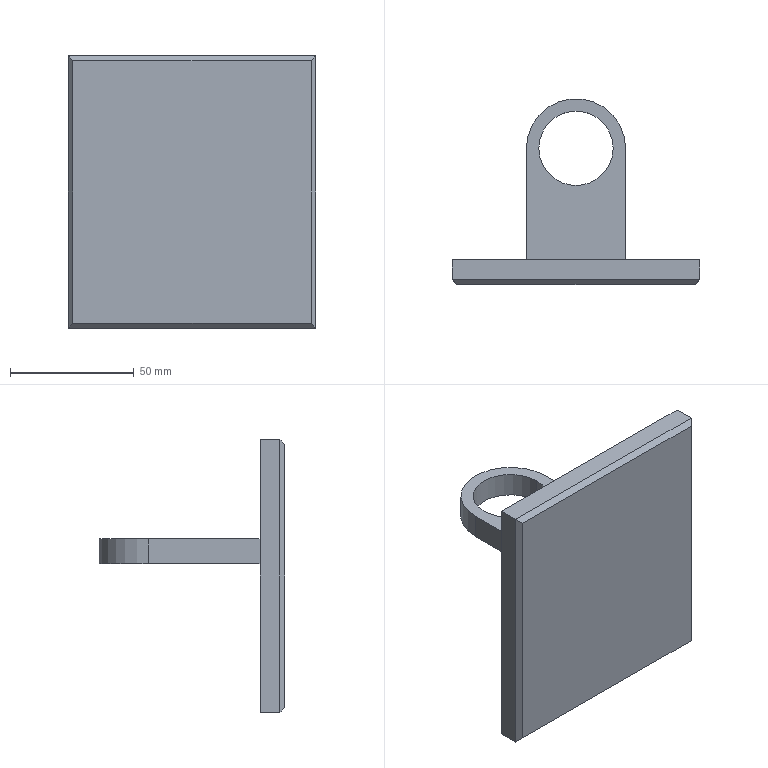Part | SolidWorks | features Chamfer 1, Extrusion 1, ICE 1 | 1 solid | 17 faces | box 100 x 75 x 110 mm | volume 126385 mm3 | plane 14 | cylinder 3 | commonest cylinder face diameters 30 x2 40 x1
STEP:
#1=CARTESIAN_POINT('',(104.,-40.,-10.));
#2=VERTEX_POINT('',#1);
#3=CARTESIAN_POINT('',(134.,-40.,-10.));
#4=VERTEX_POINT('',#3);
#5=CARTESIAN_POINT('',(119.,-40.,-10.));
#6=DIRECTION('',(0.,0.,1.));
#7=DIRECTION('',(1.,0.,0.));
#8=AXIS2_PLACEMENT_3D('',#5,#6,#7);
#9=CIRCLE('',#8,15.);
#10=EDGE_CURVE('',#2,#4,#9,.T.);
#11=ORIENTED_EDGE('',*,*,#10,.F.);
#12=CARTESIAN_POINT('',(104.,-40.,0.));
#13=VERTEX_POINT('',#12);
#14=CARTESIAN_POINT('',(104.,-40.,-10.));
#15=DIRECTION('',(0.,0.,1.));
#16=VECTOR('',#15,1000.);
#17=LINE('',#14,#16);
#18=EDGE_CURVE('',#2,#13,#17,.T.);
#19=ORIENTED_EDGE('',*,*,#18,.T.);
#20=CARTESIAN_POINT('',(134.,-40.,0.));
#21=VERTEX_POINT('',#20);
#22=CARTESIAN_POINT('',(119.,-40.,0.));
#23=DIRECTION('',(0.,0.,1.));
#24=DIRECTION('',(1.,0.,0.));
#25=AXIS2_PLACEMENT_3D('',#22,#23,#24);
#26=CIRCLE('',#25,15.);
#27=EDGE_CURVE('',#13,#21,#26,.T.);
#28=ORIENTED_EDGE('',*,*,#27,.T.);
#29=CARTESIAN_POINT('',(134.,-40.,-10.));
#30=DIRECTION('',(0.,0.,1.));
#31=VECTOR('',#30,1000.);
#32=LINE('',#29,#31);
#33=EDGE_CURVE('',#4,#21,#32,.T.);
#34=ORIENTED_EDGE('',*,*,#33,.F.);
#35=EDGE_LOOP('',(#11,#19,#28,#34));
#36=FACE_OUTER_BOUND('',#35,.T.);
#37=CARTESIAN_POINT('',(119.,-40.,-10.));
#38=DIRECTION('',(0.,0.,1.));
#39=DIRECTION('',(1.,0.,0.));
#40=AXIS2_PLACEMENT_3D('',#37,#38,#39);
#41=CYLINDRICAL_SURFACE('',#40,15.);
#42=ADVANCED_FACE('',(#36),#41,.F.);
#43=CARTESIAN_POINT('',(139.,-40.,0.));
#44=VERTEX_POINT('',#43);
#45=CARTESIAN_POINT('',(99.,-40.,0.));
#46=VERTEX_POINT('',#45);
#47=CARTESIAN_POINT('',(119.,-40.,0.));
#48=DIRECTION('',(0.,0.,1.));
#49=DIRECTION('',(1.,0.,0.));
#50=AXIS2_PLACEMENT_3D('',#47,#48,#49);
#51=CIRCLE('',#50,20.);
#52=EDGE_CURVE('',#44,#46,#51,.T.);
#53=ORIENTED_EDGE('',*,*,#52,.F.);
#54=CARTESIAN_POINT('',(139.,-40.,-10.));
#55=VERTEX_POINT('',#54);
#56=CARTESIAN_POINT('',(139.,-40.,-10.));
#57=DIRECTION('',(0.,0.,1.));
#58=VECTOR('',#57,1000.);
#59=LINE('',#56,#58);
#60=EDGE_CURVE('',#55,#44,#59,.T.);
#61=ORIENTED_EDGE('',*,*,#60,.F.);
#62=CARTESIAN_POINT('',(99.,-40.,-10.));
#63=VERTEX_POINT('',#62);
#64=CARTESIAN_POINT('',(119.,-40.,-10.));
#65=DIRECTION('',(0.,0.,1.));
#66=DIRECTION('',(1.,0.,0.));
#67=AXIS2_PLACEMENT_3D('',#64,#65,#66);
#68=CIRCLE('',#67,20.);
#69=EDGE_CURVE('',#55,#63,#68,.T.);
#70=ORIENTED_EDGE('',*,*,#69,.T.);
#71=CARTESIAN_POINT('',(99.,-40.,-10.));
#72=DIRECTION('',(0.,0.,1.));
#73=VECTOR('',#72,1000.);
#74=LINE('',#71,#73);
#75=EDGE_CURVE('',#63,#46,#74,.T.);
#76=ORIENTED_EDGE('',*,*,#75,.T.);
#77=EDGE_LOOP('',(#53,#61,#70,#76));
#78=FACE_OUTER_BOUND('',#77,.T.);
#79=CARTESIAN_POINT('',(119.,-40.,-10.));
#80=DIRECTION('',(0.,0.,1.));
#81=DIRECTION('',(1.,0.,0.));
#82=AXIS2_PLACEMENT_3D('',#79,#80,#81);
#83=CYLINDRICAL_SURFACE('',#82,20.);
#84=ADVANCED_FACE('',(#78),#83,.T.);
#85=CARTESIAN_POINT('',(139.,-85.,0.));
#86=VERTEX_POINT('',#85);
#87=CARTESIAN_POINT('',(139.,-40.,0.));
#88=DIRECTION('',(0.,1.,0.));
#89=VECTOR('',#88,1000.);
#90=LINE('',#87,#89);
#91=EDGE_CURVE('',#86,#44,#90,.T.);
#92=ORIENTED_EDGE('',*,*,#91,.F.);
#93=CARTESIAN_POINT('',(139.,-85.,-10.));
#94=VERTEX_POINT('',#93);
#95=CARTESIAN_POINT('',(139.,-85.,-10.));
#96=DIRECTION('',(0.,0.,1.));
#97=VECTOR('',#96,1000.);
#98=LINE('',#95,#97);
#99=EDGE_CURVE('',#94,#86,#98,.T.);
#100=ORIENTED_EDGE('',*,*,#99,.F.);
#101=CARTESIAN_POINT('',(139.,-40.,-10.));
#102=DIRECTION('',(0.,1.,0.));
#103=VECTOR('',#102,1000.);
#104=LINE('',#101,#103);
#105=EDGE_CURVE('',#94,#55,#104,.T.);
#106=ORIENTED_EDGE('',*,*,#105,.T.);
#107=ORIENTED_EDGE('',*,*,#60,.T.);
#108=EDGE_LOOP('',(#92,#100,#106,#107));
#109=FACE_OUTER_BOUND('',#108,.T.);
#110=CARTESIAN_POINT('',(139.,-40.,-10.));
#111=DIRECTION('',(1.,0.,0.));
#112=DIRECTION('',(0.,0.,-1.));
#113=AXIS2_PLACEMENT_3D('',#110,#111,#112);
#114=PLANE('',#113);
#115=ADVANCED_FACE('',(#109),#114,.T.);
#116=CARTESIAN_POINT('',(99.,-85.,0.));
#117=VERTEX_POINT('',#116);
#118=CARTESIAN_POINT('',(99.,-40.,0.));
#119=DIRECTION('',(0.,-1.,0.));
#120=VECTOR('',#119,1000.);
#121=LINE('',#118,#120);
#122=EDGE_CURVE('',#46,#117,#121,.T.);
#123=ORIENTED_EDGE('',*,*,#122,.F.);
#124=ORIENTED_EDGE('',*,*,#75,.F.);
#125=CARTESIAN_POINT('',(99.,-85.,-10.));
#126=VERTEX_POINT('',#125);
#127=CARTESIAN_POINT('',(99.,-40.,-10.));
#128=DIRECTION('',(0.,-1.,0.));
#129=VECTOR('',#128,1000.);
#130=LINE('',#127,#129);
#131=EDGE_CURVE('',#63,#126,#130,.T.);
#132=ORIENTED_EDGE('',*,*,#131,.T.);
#133=CARTESIAN_POINT('',(99.,-85.,-10.));
#134=DIRECTION('',(0.,0.,1.));
#135=VECTOR('',#134,1000.);
#136=LINE('',#133,#135);
#137=EDGE_CURVE('',#126,#117,#136,.T.);
#138=ORIENTED_EDGE('',*,*,#137,.T.);
#139=EDGE_LOOP('',(#123,#124,#132,#138));
#140=FACE_OUTER_BOUND('',#139,.T.);
#141=CARTESIAN_POINT('',(99.,-40.,-10.));
#142=DIRECTION('',(-1.,0.,0.));
#143=DIRECTION('',(0.,0.,1.));
#144=AXIS2_PLACEMENT_3D('',#141,#142,#143);
#145=PLANE('',#144);
#146=ADVANCED_FACE('',(#140),#145,.T.);
#147=CARTESIAN_POINT('',(119.,-40.,-10.));
#148=DIRECTION('',(0.,0.,1.));
#149=DIRECTION('',(1.,0.,0.));
#150=AXIS2_PLACEMENT_3D('',#147,#148,#149);
#151=CIRCLE('',#150,15.);
#152=EDGE_CURVE('',#4,#2,#151,.T.);
#153=ORIENTED_EDGE('',*,*,#152,.T.);
#154=ORIENTED_EDGE('',*,*,#10,.T.);
#155=EDGE_LOOP('',(#153,#154));
#156=FACE_BOUND('',#155,.T.);
#157=ORIENTED_EDGE('',*,*,#69,.F.);
#158=ORIENTED_EDGE('',*,*,#105,.F.);
#159=CARTESIAN_POINT('',(139.,-85.,-10.));
#160=DIRECTION('',(1.,0.,0.));
#161=VECTOR('',#160,1000.);
#162=LINE('',#159,#161);
#163=EDGE_CURVE('',#126,#94,#162,.T.);
#164=ORIENTED_EDGE('',*,*,#163,.F.);
#165=ORIENTED_EDGE('',*,*,#131,.F.);
#166=EDGE_LOOP('',(#157,#158,#164,#165));
#167=FACE_OUTER_BOUND('',#166,.T.);
#168=CARTESIAN_POINT('',(119.,-40.,-10.));
#169=DIRECTION('',(0.,0.,1.));
#170=DIRECTION('',(1.,0.,0.));
#171=AXIS2_PLACEMENT_3D('',#168,#169,#170);
#172=PLANE('',#171);
#173=ADVANCED_FACE('',(#156,#167),#172,.F.);
#174=CARTESIAN_POINT('',(119.,-40.,0.));
#175=DIRECTION('',(0.,0.,1.));
#176=DIRECTION('',(1.,0.,0.));
#177=AXIS2_PLACEMENT_3D('',#174,#175,#176);
#178=CIRCLE('',#177,15.);
#179=EDGE_CURVE('',#21,#13,#178,.T.);
#180=ORIENTED_EDGE('',*,*,#179,.F.);
#181=ORIENTED_EDGE('',*,*,#27,.F.);
#182=EDGE_LOOP('',(#180,#181));
#183=FACE_BOUND('',#182,.T.);
#184=ORIENTED_EDGE('',*,*,#52,.T.);
#185=ORIENTED_EDGE('',*,*,#122,.T.);
#186=CARTESIAN_POINT('',(139.,-85.,0.));
#187=DIRECTION('',(1.,0.,0.));
#188=VECTOR('',#187,1000.);
#189=LINE('',#186,#188);
#190=EDGE_CURVE('',#117,#86,#189,.T.);
#191=ORIENTED_EDGE('',*,*,#190,.T.);
#192=ORIENTED_EDGE('',*,*,#91,.T.);
#193=EDGE_LOOP('',(#184,#185,#191,#192));
#194=FACE_OUTER_BOUND('',#193,.T.);
#195=CARTESIAN_POINT('',(119.,-40.,0.));
#196=DIRECTION('',(0.,0.,1.));
#197=DIRECTION('',(1.,0.,0.));
#198=AXIS2_PLACEMENT_3D('',#195,#196,#197);
#199=PLANE('',#198);
#200=ADVANCED_FACE('',(#183,#194),#199,.T.);
#201=ORIENTED_EDGE('',*,*,#18,.F.);
#202=ORIENTED_EDGE('',*,*,#152,.F.);
#203=ORIENTED_EDGE('',*,*,#33,.T.);
#204=ORIENTED_EDGE('',*,*,#179,.T.);
#205=EDGE_LOOP('',(#201,#202,#203,#204));
#206=FACE_OUTER_BOUND('',#205,.T.);
#207=CARTESIAN_POINT('',(119.,-40.,-10.));
#208=DIRECTION('',(0.,0.,1.));
#209=DIRECTION('',(1.,0.,0.));
#210=AXIS2_PLACEMENT_3D('',#207,#208,#209);
#211=CYLINDRICAL_SURFACE('',#210,15.);
#212=ADVANCED_FACE('',(#206),#211,.F.);
#213=CARTESIAN_POINT('',(169.,-93.,40.));
#214=VERTEX_POINT('',#213);
#215=CARTESIAN_POINT('',(169.,-85.,40.));
#216=VERTEX_POINT('',#215);
#217=CARTESIAN_POINT('',(169.,-95.,40.));
#218=DIRECTION('',(0.,1.,0.));
#219=VECTOR('',#218,1000.);
#220=LINE('',#217,#219);
#221=EDGE_CURVE('',#214,#216,#220,.T.);
#222=ORIENTED_EDGE('',*,*,#221,.F.);
#223=CARTESIAN_POINT('',(169.,-93.,-70.));
#224=VERTEX_POINT('',#223);
#225=CARTESIAN_POINT('',(169.,-93.,-70.));
#226=DIRECTION('',(0.,0.,-1.));
#227=VECTOR('',#226,1000.);
#228=LINE('',#225,#227);
#229=EDGE_CURVE('',#214,#224,#228,.T.);
#230=ORIENTED_EDGE('',*,*,#229,.T.);
#231=CARTESIAN_POINT('',(169.,-85.,-70.));
#232=VERTEX_POINT('',#231);
#233=CARTESIAN_POINT('',(169.,-95.,-70.));
#234=DIRECTION('',(0.,1.,0.));
#235=VECTOR('',#234,1000.);
#236=LINE('',#233,#235);
#237=EDGE_CURVE('',#224,#232,#236,.T.);
#238=ORIENTED_EDGE('',*,*,#237,.T.);
#239=CARTESIAN_POINT('',(169.,-85.,-70.));
#240=DIRECTION('',(0.,0.,1.));
#241=VECTOR('',#240,1000.);
#242=LINE('',#239,#241);
#243=EDGE_CURVE('',#232,#216,#242,.T.);
#244=ORIENTED_EDGE('',*,*,#243,.T.);
#245=EDGE_LOOP('',(#222,#230,#238,#244));
#246=FACE_OUTER_BOUND('',#245,.T.);
#247=CARTESIAN_POINT('',(169.,-95.,-70.));
#248=DIRECTION('',(-1.,0.,0.));
#249=DIRECTION('',(0.,0.,1.));
#250=AXIS2_PLACEMENT_3D('',#247,#248,#249);
#251=PLANE('',#250);
#252=ADVANCED_FACE('',(#246),#251,.F.);
#253=CARTESIAN_POINT('',(69.,-93.,40.));
#254=VERTEX_POINT('',#253);
#255=CARTESIAN_POINT('',(69.,-85.,40.));
#256=VERTEX_POINT('',#255);
#257=CARTESIAN_POINT('',(69.,-95.,40.));
#258=DIRECTION('',(0.,1.,0.));
#259=VECTOR('',#258,1000.);
#260=LINE('',#257,#259);
#261=EDGE_CURVE('',#254,#256,#260,.T.);
#262=ORIENTED_EDGE('',*,*,#261,.F.);
#263=CARTESIAN_POINT('',(169.,-93.,40.));
#264=DIRECTION('',(1.,0.,0.));
#265=VECTOR('',#264,1000.);
#266=LINE('',#263,#265);
#267=EDGE_CURVE('',#254,#214,#266,.T.);
#268=ORIENTED_EDGE('',*,*,#267,.T.);
#269=ORIENTED_EDGE('',*,*,#221,.T.);
#270=CARTESIAN_POINT('',(169.,-85.,40.));
#271=DIRECTION('',(-1.,0.,0.));
#272=VECTOR('',#271,1000.);
#273=LINE('',#270,#272);
#274=EDGE_CURVE('',#216,#256,#273,.T.);
#275=ORIENTED_EDGE('',*,*,#274,.T.);
#276=EDGE_LOOP('',(#262,#268,#269,#275));
#277=FACE_OUTER_BOUND('',#276,.T.);
#278=CARTESIAN_POINT('',(169.,-95.,40.));
#279=DIRECTION('',(0.,0.,-1.));
#280=DIRECTION('',(-1.,0.,0.));
#281=AXIS2_PLACEMENT_3D('',#278,#279,#280);
#282=PLANE('',#281);
#283=ADVANCED_FACE('',(#277),#282,.F.);
#284=CARTESIAN_POINT('',(69.,-93.,-70.));
#285=VERTEX_POINT('',#284);
#286=CARTESIAN_POINT('',(69.,-85.,-70.));
#287=VERTEX_POINT('',#286);
#288=CARTESIAN_POINT('',(69.,-95.,-70.));
#289=DIRECTION('',(0.,1.,0.));
#290=VECTOR('',#289,1000.);
#291=LINE('',#288,#290);
#292=EDGE_CURVE('',#285,#287,#291,.T.);
#293=ORIENTED_EDGE('',*,*,#292,.F.);
#294=CARTESIAN_POINT('',(69.,-93.,40.));
#295=DIRECTION('',(0.,0.,1.));
#296=VECTOR('',#295,1000.);
#297=LINE('',#294,#296);
#298=EDGE_CURVE('',#285,#254,#297,.T.);
#299=ORIENTED_EDGE('',*,*,#298,.T.);
#300=ORIENTED_EDGE('',*,*,#261,.T.);
#301=CARTESIAN_POINT('',(69.,-85.,-70.));
#302=DIRECTION('',(0.,0.,-1.));
#303=VECTOR('',#302,1000.);
#304=LINE('',#301,#303);
#305=EDGE_CURVE('',#256,#287,#304,.T.);
#306=ORIENTED_EDGE('',*,*,#305,.T.);
#307=EDGE_LOOP('',(#293,#299,#300,#306));
#308=FACE_OUTER_BOUND('',#307,.T.);
#309=CARTESIAN_POINT('',(69.,-95.,-70.));
#310=DIRECTION('',(1.,0.,0.));
#311=DIRECTION('',(0.,0.,-1.));
#312=AXIS2_PLACEMENT_3D('',#309,#310,#311);
#313=PLANE('',#312);
#314=ADVANCED_FACE('',(#308),#313,.F.);
#315=ORIENTED_EDGE('',*,*,#237,.F.);
#316=CARTESIAN_POINT('',(69.,-93.,-70.));
#317=DIRECTION('',(-1.,0.,0.));
#318=VECTOR('',#317,1000.);
#319=LINE('',#316,#318);
#320=EDGE_CURVE('',#224,#285,#319,.T.);
#321=ORIENTED_EDGE('',*,*,#320,.T.);
#322=ORIENTED_EDGE('',*,*,#292,.T.);
#323=CARTESIAN_POINT('',(169.,-85.,-70.));
#324=DIRECTION('',(1.,0.,0.));
#325=VECTOR('',#324,1000.);
#326=LINE('',#323,#325);
#327=EDGE_CURVE('',#287,#232,#326,.T.);
#328=ORIENTED_EDGE('',*,*,#327,.T.);
#329=EDGE_LOOP('',(#315,#321,#322,#328));
#330=FACE_OUTER_BOUND('',#329,.T.);
#331=CARTESIAN_POINT('',(169.,-95.,-70.));
#332=DIRECTION('',(0.,0.,1.));
#333=DIRECTION('',(1.,0.,0.));
#334=AXIS2_PLACEMENT_3D('',#331,#332,#333);
#335=PLANE('',#334);
#336=ADVANCED_FACE('',(#330),#335,.F.);
#337=CARTESIAN_POINT('',(71.,-95.,38.));
#338=VERTEX_POINT('',#337);
#339=CARTESIAN_POINT('',(71.,-95.,-68.));
#340=VERTEX_POINT('',#339);
#341=CARTESIAN_POINT('',(71.,-95.,-70.));
#342=DIRECTION('',(0.,0.,-1.));
#343=VECTOR('',#342,1000.);
#344=LINE('',#341,#343);
#345=EDGE_CURVE('',#338,#340,#344,.T.);
#346=ORIENTED_EDGE('',*,*,#345,.T.);
#347=CARTESIAN_POINT('',(167.,-95.,-68.));
#348=VERTEX_POINT('',#347);
#349=CARTESIAN_POINT('',(169.,-95.,-68.));
#350=DIRECTION('',(1.,0.,0.));
#351=VECTOR('',#350,1000.);
#352=LINE('',#349,#351);
#353=EDGE_CURVE('',#340,#348,#352,.T.);
#354=ORIENTED_EDGE('',*,*,#353,.T.);
#355=CARTESIAN_POINT('',(167.,-95.,38.));
#356=VERTEX_POINT('',#355);
#357=CARTESIAN_POINT('',(167.,-95.,40.));
#358=DIRECTION('',(0.,0.,1.));
#359=VECTOR('',#358,1000.);
#360=LINE('',#357,#359);
#361=EDGE_CURVE('',#348,#356,#360,.T.);
#362=ORIENTED_EDGE('',*,*,#361,.T.);
#363=CARTESIAN_POINT('',(69.,-95.,38.));
#364=DIRECTION('',(-1.,0.,0.));
#365=VECTOR('',#364,1000.);
#366=LINE('',#363,#365);
#367=EDGE_CURVE('',#356,#338,#366,.T.);
#368=ORIENTED_EDGE('',*,*,#367,.T.);
#369=EDGE_LOOP('',(#346,#354,#362,#368));
#370=FACE_OUTER_BOUND('',#369,.T.);
#371=CARTESIAN_POINT('',(0.,-95.,0.));
#372=DIRECTION('',(0.,-1.,0.));
#373=DIRECTION('',(0.,0.,-1.));
#374=AXIS2_PLACEMENT_3D('',#371,#372,#373);
#375=PLANE('',#374);
#376=ADVANCED_FACE('',(#370),#375,.T.);
#377=ORIENTED_EDGE('',*,*,#190,.F.);
#378=ORIENTED_EDGE('',*,*,#137,.F.);
#379=ORIENTED_EDGE('',*,*,#163,.T.);
#380=ORIENTED_EDGE('',*,*,#99,.T.);
#381=EDGE_LOOP('',(#377,#378,#379,#380));
#382=FACE_BOUND('',#381,.T.);
#383=ORIENTED_EDGE('',*,*,#243,.F.);
#384=ORIENTED_EDGE('',*,*,#327,.F.);
#385=ORIENTED_EDGE('',*,*,#305,.F.);
#386=ORIENTED_EDGE('',*,*,#274,.F.);
#387=EDGE_LOOP('',(#383,#384,#385,#386));
#388=FACE_OUTER_BOUND('',#387,.T.);
#389=CARTESIAN_POINT('',(0.,-85.,0.));
#390=DIRECTION('',(0.,-1.,0.));
#391=DIRECTION('',(0.,0.,-1.));
#392=AXIS2_PLACEMENT_3D('',#389,#390,#391);
#393=PLANE('',#392);
#394=ADVANCED_FACE('',(#382,#388),#393,.F.);
#395=CARTESIAN_POINT('',(154.333,-107.667,25.333));
#396=DIRECTION('',(-0.5774,-0.5774,-0.5774));
#397=VECTOR('',#396,1000.);
#398=LINE('',#395,#397);
#399=EDGE_CURVE('',#214,#356,#398,.T.);
#400=ORIENTED_EDGE('',*,*,#399,.F.);
#401=ORIENTED_EDGE('',*,*,#267,.F.);
#402=CARTESIAN_POINT('',(47.333,-71.333,61.667));
#403=DIRECTION('',(-0.5774,0.5774,0.5774));
#404=VECTOR('',#403,1000.);
#405=LINE('',#402,#404);
#406=EDGE_CURVE('',#338,#254,#405,.T.);
#407=ORIENTED_EDGE('',*,*,#406,.F.);
#408=ORIENTED_EDGE('',*,*,#367,.F.);
#409=EDGE_LOOP('',(#400,#401,#407,#408));
#410=FACE_OUTER_BOUND('',#409,.T.);
#411=CARTESIAN_POINT('',(0.,-95.,38.));
#412=DIRECTION('',(0.,-0.7071,0.7071));
#413=DIRECTION('',(1.,0.,0.));
#414=AXIS2_PLACEMENT_3D('',#411,#412,#413);
#415=PLANE('',#414);
#416=ADVANCED_FACE('',(#410),#415,.T.);
#417=ORIENTED_EDGE('',*,*,#406,.T.);
#418=ORIENTED_EDGE('',*,*,#298,.F.);
#419=CARTESIAN_POINT('',(93.667,-117.667,-45.333));
#420=DIRECTION('',(-0.5774,0.5774,-0.5774));
#421=VECTOR('',#420,1000.);
#422=LINE('',#419,#421);
#423=EDGE_CURVE('',#340,#285,#422,.T.);
#424=ORIENTED_EDGE('',*,*,#423,.F.);
#425=ORIENTED_EDGE('',*,*,#345,.F.);
#426=EDGE_LOOP('',(#417,#418,#424,#425));
#427=FACE_OUTER_BOUND('',#426,.T.);
#428=CARTESIAN_POINT('',(71.,-95.,0.));
#429=DIRECTION('',(-0.7071,-0.7071,0.));
#430=DIRECTION('',(0.,0.,1.));
#431=AXIS2_PLACEMENT_3D('',#428,#429,#430);
#432=PLANE('',#431);
#433=ADVANCED_FACE('',(#427),#432,.T.);
#434=ORIENTED_EDGE('',*,*,#399,.T.);
#435=ORIENTED_EDGE('',*,*,#361,.F.);
#436=CARTESIAN_POINT('',(144.333,-117.667,-45.333));
#437=DIRECTION('',(-0.5774,-0.5774,0.5774));
#438=VECTOR('',#437,1000.);
#439=LINE('',#436,#438);
#440=EDGE_CURVE('',#224,#348,#439,.T.);
#441=ORIENTED_EDGE('',*,*,#440,.F.);
#442=ORIENTED_EDGE('',*,*,#229,.F.);
#443=EDGE_LOOP('',(#434,#435,#441,#442));
#444=FACE_OUTER_BOUND('',#443,.T.);
#445=CARTESIAN_POINT('',(167.,-95.,0.));
#446=DIRECTION('',(0.7071,-0.7071,0.));
#447=DIRECTION('',(0.,0.,-1.));
#448=AXIS2_PLACEMENT_3D('',#445,#446,#447);
#449=PLANE('',#448);
#450=ADVANCED_FACE('',(#444),#449,.T.);
#451=ORIENTED_EDGE('',*,*,#423,.T.);
#452=ORIENTED_EDGE('',*,*,#320,.F.);
#453=ORIENTED_EDGE('',*,*,#440,.T.);
#454=ORIENTED_EDGE('',*,*,#353,.F.);
#455=EDGE_LOOP('',(#451,#452,#453,#454));
#456=FACE_OUTER_BOUND('',#455,.T.);
#457=CARTESIAN_POINT('',(0.,-95.,-68.));
#458=DIRECTION('',(0.,-0.7071,-0.7071));
#459=DIRECTION('',(-1.,0.,0.));
#460=AXIS2_PLACEMENT_3D('',#457,#458,#459);
#461=PLANE('',#460);
#462=ADVANCED_FACE('',(#456),#461,.T.);
#463=CLOSED_SHELL('',(#42,#84,#115,#146,#173,#200,#212,#252,#283,#314,#336,#376,#394,#416,#433,#450,#462));
#464=MANIFOLD_SOLID_BREP('',#463);
#465=CARTESIAN_POINT('',(0.,0.,0.));
#466=DIRECTION('',(0.,0.,1.));
#467=DIRECTION('',(1.,0.,0.));
#468=AXIS2_PLACEMENT_3D('',#465,#466,#467);
#469=(LENGTH_UNIT()NAMED_UNIT(*)SI_UNIT(.MILLI.,.METRE.));
#470=UNCERTAINTY_MEASURE_WITH_UNIT(LENGTH_MEASURE(0.00001),#469,'','');
#471=(NAMED_UNIT(*)PLANE_ANGLE_UNIT()SI_UNIT($,.RADIAN.));
#472=(NAMED_UNIT(*)SI_UNIT($,.STERADIAN.)SOLID_ANGLE_UNIT());
#473=(GEOMETRIC_REPRESENTATION_CONTEXT(3)GLOBAL_UNCERTAINTY_ASSIGNED_CONTEXT((#470))GLOBAL_UNIT_ASSIGNED_CONTEXT((#469,#471,#472))REPRESENTATION_CONTEXT('',''));
#474=ADVANCED_BREP_SHAPE_REPRESENTATION('',(#464,#468),#473);